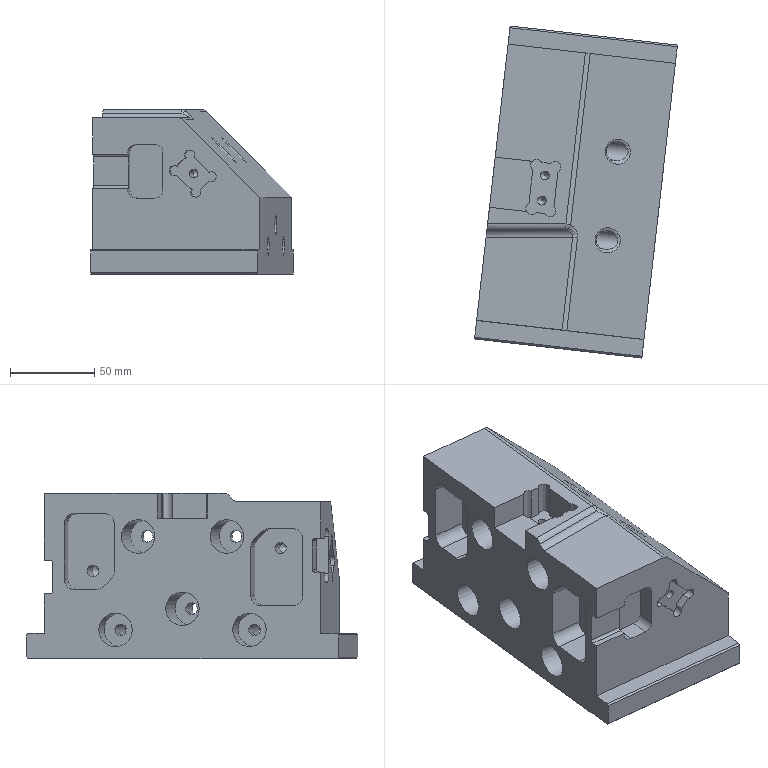Part | NX | features XQ 2 | 1 solid | 141 faces | box 120.526 x 197.118 x 98 mm | volume 1230326 mm3 | plane 72 | cylinder 59 | cone 6 | spline 3 | sphere 1 | commonest cylinder face diameters 12 x10 7 x9 10 x9 6 x8 11 x5 20 x5